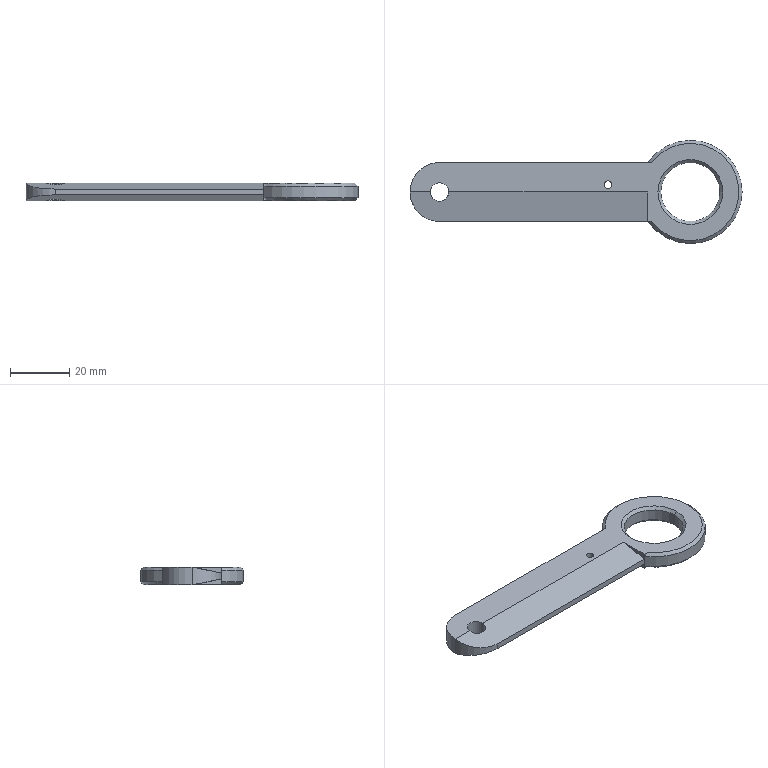Part | SolidWorks | features ICE 3, Chamfer 1, Extrusion 1, HoleWzd 1 | 1 solid | 24 faces | box 112.5 x 35 x 6 mm | volume 11153 mm3 | cylinder 9 | plane 8 | cone 7 | commonest cylinder face diameters 20 x4 2.5 x2 6.2 x2 35 x1
STEP:
#1=CARTESIAN_POINT('',(13.362,2.5,6.));
#2=VERTEX_POINT('',#1);
#3=CARTESIAN_POINT('',(15.862,2.5,6.));
#4=VERTEX_POINT('',#3);
#5=CARTESIAN_POINT('',(14.612,2.5,6.));
#6=DIRECTION('',(0.,0.,1.));
#7=DIRECTION('',(1.,0.,0.));
#8=AXIS2_PLACEMENT_3D('',#5,#6,#7);
#9=CIRCLE('',#8,1.25);
#10=EDGE_CURVE('',#2,#4,#9,.T.);
#11=ORIENTED_EDGE('',*,*,#10,.T.);
#12=CARTESIAN_POINT('',(15.862,2.5,0.));
#13=VERTEX_POINT('',#12);
#14=CARTESIAN_POINT('',(15.862,2.5,0.));
#15=DIRECTION('',(0.,0.,-1.));
#16=VECTOR('',#15,1000.);
#17=LINE('',#14,#16);
#18=EDGE_CURVE('',#4,#13,#17,.T.);
#19=ORIENTED_EDGE('',*,*,#18,.T.);
#20=CARTESIAN_POINT('',(13.362,2.5,0.));
#21=VERTEX_POINT('',#20);
#22=CARTESIAN_POINT('',(14.612,2.5,0.));
#23=DIRECTION('',(0.,0.,-1.));
#24=DIRECTION('',(-1.,0.,0.));
#25=AXIS2_PLACEMENT_3D('',#22,#23,#24);
#26=CIRCLE('',#25,1.25);
#27=EDGE_CURVE('',#13,#21,#26,.T.);
#28=ORIENTED_EDGE('',*,*,#27,.T.);
#29=CARTESIAN_POINT('',(13.362,2.5,0.));
#30=DIRECTION('',(0.,0.,-1.));
#31=VECTOR('',#30,1000.);
#32=LINE('',#29,#31);
#33=EDGE_CURVE('',#2,#21,#32,.T.);
#34=ORIENTED_EDGE('',*,*,#33,.F.);
#35=EDGE_LOOP('',(#11,#19,#28,#34));
#36=FACE_OUTER_BOUND('',#35,.T.);
#37=CARTESIAN_POINT('',(14.612,2.5,0.));
#38=DIRECTION('',(0.,0.,-1.));
#39=DIRECTION('',(-1.,0.,0.));
#40=AXIS2_PLACEMENT_3D('',#37,#38,#39);
#41=CYLINDRICAL_SURFACE('',#40,1.25);
#42=ADVANCED_FACE('',(#36),#41,.F.);
#43=CARTESIAN_POINT('',(52.5,0.,1.));
#44=VERTEX_POINT('',#43);
#45=CARTESIAN_POINT('',(32.5,0.,1.));
#46=VERTEX_POINT('',#45);
#47=CARTESIAN_POINT('',(42.5,0.,1.));
#48=DIRECTION('',(0.,0.,-1.));
#49=DIRECTION('',(1.,0.,0.));
#50=AXIS2_PLACEMENT_3D('',#47,#48,#49);
#51=CIRCLE('',#50,10.);
#52=EDGE_CURVE('',#44,#46,#51,.T.);
#53=ORIENTED_EDGE('',*,*,#52,.F.);
#54=CARTESIAN_POINT('',(53.5,0.,0.));
#55=VERTEX_POINT('',#54);
#56=CARTESIAN_POINT('',(52.5,0.,1.));
#57=DIRECTION('',(0.7071,0.,-0.7071));
#58=VECTOR('',#57,1000.);
#59=LINE('',#56,#58);
#60=EDGE_CURVE('',#44,#55,#59,.T.);
#61=ORIENTED_EDGE('',*,*,#60,.T.);
#62=CARTESIAN_POINT('',(31.5,0.,0.));
#63=VERTEX_POINT('',#62);
#64=CARTESIAN_POINT('',(42.5,0.,0.));
#65=DIRECTION('',(0.,0.,1.));
#66=DIRECTION('',(1.,0.,0.));
#67=AXIS2_PLACEMENT_3D('',#64,#65,#66);
#68=CIRCLE('',#67,11.);
#69=EDGE_CURVE('',#63,#55,#68,.T.);
#70=ORIENTED_EDGE('',*,*,#69,.F.);
#71=CARTESIAN_POINT('',(32.5,0.,1.));
#72=DIRECTION('',(-0.7071,0.,-0.7071));
#73=VECTOR('',#72,1000.);
#74=LINE('',#71,#73);
#75=EDGE_CURVE('',#46,#63,#74,.T.);
#76=ORIENTED_EDGE('',*,*,#75,.F.);
#77=EDGE_LOOP('',(#53,#61,#70,#76));
#78=FACE_OUTER_BOUND('',#77,.T.);
#79=CARTESIAN_POINT('',(42.5,0.,1.));
#80=DIRECTION('',(0.,0.,-1.));
#81=DIRECTION('',(-1.,0.,0.));
#82=AXIS2_PLACEMENT_3D('',#79,#80,#81);
#83=CONICAL_SURFACE('',#82,10.,0.7854);
#84=ADVANCED_FACE('',(#78),#83,.F.);
#85=CARTESIAN_POINT('',(59.,0.,0.));
#86=VERTEX_POINT('',#85);
#87=CARTESIAN_POINT('',(29.376,-10.,0.));
#88=VERTEX_POINT('',#87);
#89=CARTESIAN_POINT('',(42.5,0.,0.));
#90=DIRECTION('',(0.,0.,-1.));
#91=DIRECTION('',(1.,0.,0.));
#92=AXIS2_PLACEMENT_3D('',#89,#90,#91);
#93=CIRCLE('',#92,16.5);
#94=EDGE_CURVE('',#86,#88,#93,.T.);
#95=ORIENTED_EDGE('',*,*,#94,.F.);
#96=CARTESIAN_POINT('',(60.,0.,1.));
#97=VERTEX_POINT('',#96);
#98=CARTESIAN_POINT('',(60.,0.,1.));
#99=DIRECTION('',(0.7071,0.,0.7071));
#100=VECTOR('',#99,1000.);
#101=LINE('',#98,#100);
#102=EDGE_CURVE('',#86,#97,#101,.T.);
#103=ORIENTED_EDGE('',*,*,#102,.T.);
#104=CARTESIAN_POINT('',(28.139,-10.,1.));
#105=VERTEX_POINT('',#104);
#106=CARTESIAN_POINT('',(42.5,0.,1.));
#107=DIRECTION('',(0.,0.,1.));
#108=DIRECTION('',(1.,0.,0.));
#109=AXIS2_PLACEMENT_3D('',#106,#107,#108);
#110=CIRCLE('',#109,17.5);
#111=EDGE_CURVE('',#105,#97,#110,.T.);
#112=ORIENTED_EDGE('',*,*,#111,.F.);
#113=CARTESIAN_POINT('',(29.376,-10.,0.));
#114=CARTESIAN_POINT('',(28.961,-10.,0.3301));
#115=CARTESIAN_POINT('',(28.548,-10.,0.6636));
#116=CARTESIAN_POINT('',(28.139,-10.,1.));
#117=B_SPLINE_CURVE_WITH_KNOTS('',3,(#113,#114,#115,#116),.UNSPECIFIED.,.F.,.F.,(4,4),(0.,0.001591),.UNSPECIFIED.);
#118=EDGE_CURVE('',#88,#105,#117,.T.);
#119=ORIENTED_EDGE('',*,*,#118,.F.);
#120=EDGE_LOOP('',(#95,#103,#112,#119));
#121=FACE_OUTER_BOUND('',#120,.T.);
#122=CARTESIAN_POINT('',(42.5,0.,1.));
#123=DIRECTION('',(0.,0.,1.));
#124=DIRECTION('',(1.,0.,0.));
#125=AXIS2_PLACEMENT_3D('',#122,#123,#124);
#126=CONICAL_SURFACE('',#125,17.5,0.7854);
#127=ADVANCED_FACE('',(#121),#126,.T.);
#128=CARTESIAN_POINT('',(32.5,0.,5.));
#129=VERTEX_POINT('',#128);
#130=CARTESIAN_POINT('',(52.5,0.,5.));
#131=VERTEX_POINT('',#130);
#132=CARTESIAN_POINT('',(42.5,0.,5.));
#133=DIRECTION('',(0.,0.,1.));
#134=DIRECTION('',(1.,0.,0.));
#135=AXIS2_PLACEMENT_3D('',#132,#133,#134);
#136=CIRCLE('',#135,10.);
#137=EDGE_CURVE('',#129,#131,#136,.T.);
#138=ORIENTED_EDGE('',*,*,#137,.F.);
#139=CARTESIAN_POINT('',(31.5,0.,6.));
#140=VERTEX_POINT('',#139);
#141=CARTESIAN_POINT('',(32.5,0.,5.));
#142=DIRECTION('',(-0.7071,0.,0.7071));
#143=VECTOR('',#142,1000.);
#144=LINE('',#141,#143);
#145=EDGE_CURVE('',#129,#140,#144,.T.);
#146=ORIENTED_EDGE('',*,*,#145,.T.);
#147=CARTESIAN_POINT('',(53.5,0.,6.));
#148=VERTEX_POINT('',#147);
#149=CARTESIAN_POINT('',(42.5,0.,6.));
#150=DIRECTION('',(0.,0.,-1.));
#151=DIRECTION('',(1.,0.,0.));
#152=AXIS2_PLACEMENT_3D('',#149,#150,#151);
#153=CIRCLE('',#152,11.);
#154=EDGE_CURVE('',#148,#140,#153,.T.);
#155=ORIENTED_EDGE('',*,*,#154,.F.);
#156=CARTESIAN_POINT('',(52.5,0.,5.));
#157=DIRECTION('',(0.7071,0.,0.7071));
#158=VECTOR('',#157,1000.);
#159=LINE('',#156,#158);
#160=EDGE_CURVE('',#131,#148,#159,.T.);
#161=ORIENTED_EDGE('',*,*,#160,.F.);
#162=EDGE_LOOP('',(#138,#146,#155,#161));
#163=FACE_OUTER_BOUND('',#162,.T.);
#164=CARTESIAN_POINT('',(42.5,0.,5.));
#165=DIRECTION('',(0.,0.,1.));
#166=DIRECTION('',(1.,0.,0.));
#167=AXIS2_PLACEMENT_3D('',#164,#165,#166);
#168=CONICAL_SURFACE('',#167,10.,0.7854);
#169=ADVANCED_FACE('',(#163),#168,.F.);
#170=CARTESIAN_POINT('',(-45.6,0.,6.));
#171=VERTEX_POINT('',#170);
#172=CARTESIAN_POINT('',(-39.4,0.,6.));
#173=VERTEX_POINT('',#172);
#174=CARTESIAN_POINT('',(-45.6,0.,6.));
#175=CARTESIAN_POINT('',(-45.6,-6.2,4.76));
#176=CARTESIAN_POINT('',(-39.4,-6.2,4.76));
#177=CARTESIAN_POINT('',(-39.4,0.,6.));
#178=(BOUNDED_CURVE()B_SPLINE_CURVE(3,(#174,#175,#176,#177),.UNSPECIFIED.,.F.,.F.)B_SPLINE_CURVE_WITH_KNOTS((4,4),(4.712,7.854),.UNSPECIFIED.)CURVE()GEOMETRIC_REPRESENTATION_ITEM()RATIONAL_B_SPLINE_CURVE((1.,0.3333,0.3333,1.))REPRESENTATION_ITEM(''));
#179=EDGE_CURVE('',#171,#173,#178,.T.);
#180=ORIENTED_EDGE('',*,*,#179,.T.);
#181=CARTESIAN_POINT('',(-39.4,0.,0.));
#182=VERTEX_POINT('',#181);
#183=CARTESIAN_POINT('',(-39.4,0.,10.));
#184=DIRECTION('',(0.,0.,-1.));
#185=VECTOR('',#184,1000.);
#186=LINE('',#183,#185);
#187=EDGE_CURVE('',#173,#182,#186,.T.);
#188=ORIENTED_EDGE('',*,*,#187,.T.);
#189=CARTESIAN_POINT('',(-45.6,0.,0.));
#190=VERTEX_POINT('',#189);
#191=CARTESIAN_POINT('',(-39.4,0.,0.));
#192=CARTESIAN_POINT('',(-39.4,-6.2,1.24));
#193=CARTESIAN_POINT('',(-45.6,-6.2,1.24));
#194=CARTESIAN_POINT('',(-45.6,0.,0.));
#195=(BOUNDED_CURVE()B_SPLINE_CURVE(3,(#191,#192,#193,#194),.UNSPECIFIED.,.F.,.F.)B_SPLINE_CURVE_WITH_KNOTS((4,4),(1.571,4.712),.UNSPECIFIED.)CURVE()GEOMETRIC_REPRESENTATION_ITEM()RATIONAL_B_SPLINE_CURVE((1.,0.3333,0.3333,1.))REPRESENTATION_ITEM(''));
#196=EDGE_CURVE('',#182,#190,#195,.T.);
#197=ORIENTED_EDGE('',*,*,#196,.T.);
#198=CARTESIAN_POINT('',(-45.6,0.,10.));
#199=DIRECTION('',(0.,0.,-1.));
#200=VECTOR('',#199,1000.);
#201=LINE('',#198,#200);
#202=EDGE_CURVE('',#171,#190,#201,.T.);
#203=ORIENTED_EDGE('',*,*,#202,.F.);
#204=EDGE_LOOP('',(#180,#188,#197,#203));
#205=FACE_OUTER_BOUND('',#204,.T.);
#206=CARTESIAN_POINT('',(-42.5,0.,10.));
#207=DIRECTION('',(0.,0.,-1.));
#208=DIRECTION('',(-1.,0.,0.));
#209=AXIS2_PLACEMENT_3D('',#206,#207,#208);
#210=CYLINDRICAL_SURFACE('',#209,3.1);
#211=ADVANCED_FACE('',(#205),#210,.F.);
#212=ORIENTED_EDGE('',*,*,#137,.T.);
#213=CARTESIAN_POINT('',(52.5,0.,10.));
#214=DIRECTION('',(0.,0.,-1.));
#215=VECTOR('',#214,1000.);
#216=LINE('',#213,#215);
#217=EDGE_CURVE('',#131,#44,#216,.T.);
#218=ORIENTED_EDGE('',*,*,#217,.T.);
#219=ORIENTED_EDGE('',*,*,#52,.T.);
#220=CARTESIAN_POINT('',(32.5,0.,10.));
#221=DIRECTION('',(0.,0.,-1.));
#222=VECTOR('',#221,1000.);
#223=LINE('',#220,#222);
#224=EDGE_CURVE('',#129,#46,#223,.T.);
#225=ORIENTED_EDGE('',*,*,#224,.F.);
#226=EDGE_LOOP('',(#212,#218,#219,#225));
#227=FACE_OUTER_BOUND('',#226,.T.);
#228=CARTESIAN_POINT('',(42.5,0.,10.));
#229=DIRECTION('',(0.,0.,-1.));
#230=DIRECTION('',(-1.,0.,0.));
#231=AXIS2_PLACEMENT_3D('',#228,#229,#230);
#232=CYLINDRICAL_SURFACE('',#231,10.);
#233=ADVANCED_FACE('',(#227),#232,.F.);
#234=CARTESIAN_POINT('',(-42.5,-10.,4.));
#235=VERTEX_POINT('',#234);
#236=CARTESIAN_POINT('',(-52.5,0.,6.));
#237=VERTEX_POINT('',#236);
#238=CARTESIAN_POINT('',(-42.5,-10.,4.));
#239=CARTESIAN_POINT('',(-48.358,-10.,4.));
#240=CARTESIAN_POINT('',(-52.5,-5.858,4.828));
#241=CARTESIAN_POINT('',(-52.5,0.,6.));
#242=(BOUNDED_CURVE()B_SPLINE_CURVE(3,(#238,#239,#240,#241),.UNSPECIFIED.,.F.,.F.)B_SPLINE_CURVE_WITH_KNOTS((4,4),(0.,1.571),.UNSPECIFIED.)CURVE()GEOMETRIC_REPRESENTATION_ITEM()RATIONAL_B_SPLINE_CURVE((1.,0.8047,0.8047,1.))REPRESENTATION_ITEM(''));
#243=EDGE_CURVE('',#235,#237,#242,.T.);
#244=ORIENTED_EDGE('',*,*,#243,.T.);
#245=CARTESIAN_POINT('',(-52.5,0.,0.));
#246=VERTEX_POINT('',#245);
#247=CARTESIAN_POINT('',(-52.5,0.,6.));
#248=DIRECTION('',(0.,0.,-1.));
#249=VECTOR('',#248,1000.);
#250=LINE('',#247,#249);
#251=EDGE_CURVE('',#237,#246,#250,.T.);
#252=ORIENTED_EDGE('',*,*,#251,.T.);
#253=CARTESIAN_POINT('',(-42.5,-10.,2.));
#254=VERTEX_POINT('',#253);
#255=CARTESIAN_POINT('',(-52.5,0.,0.));
#256=CARTESIAN_POINT('',(-52.5,-5.858,1.172));
#257=CARTESIAN_POINT('',(-48.358,-10.,2.));
#258=CARTESIAN_POINT('',(-42.5,-10.,2.));
#259=(BOUNDED_CURVE()B_SPLINE_CURVE(3,(#255,#256,#257,#258),.UNSPECIFIED.,.F.,.F.)B_SPLINE_CURVE_WITH_KNOTS((4,4),(1.571,3.142),.UNSPECIFIED.)CURVE()GEOMETRIC_REPRESENTATION_ITEM()RATIONAL_B_SPLINE_CURVE((1.,0.8047,0.8047,1.))REPRESENTATION_ITEM(''));
#260=EDGE_CURVE('',#246,#254,#259,.T.);
#261=ORIENTED_EDGE('',*,*,#260,.T.);
#262=CARTESIAN_POINT('',(-42.5,-10.,6.));
#263=DIRECTION('',(0.,0.,-1.));
#264=VECTOR('',#263,1000.);
#265=LINE('',#262,#264);
#266=EDGE_CURVE('',#235,#254,#265,.T.);
#267=ORIENTED_EDGE('',*,*,#266,.F.);
#268=EDGE_LOOP('',(#244,#252,#261,#267));
#269=FACE_OUTER_BOUND('',#268,.T.);
#270=CARTESIAN_POINT('',(-42.5,0.,6.));
#271=DIRECTION('',(0.,0.,-1.));
#272=DIRECTION('',(-1.,0.,0.));
#273=AXIS2_PLACEMENT_3D('',#270,#271,#272);
#274=CYLINDRICAL_SURFACE('',#273,10.);
#275=ADVANCED_FACE('',(#269),#274,.T.);
#276=CARTESIAN_POINT('',(28.,-10.,6.));
#277=VERTEX_POINT('',#276);
#278=CARTESIAN_POINT('',(28.,-10.,4.));
#279=VERTEX_POINT('',#278);
#280=CARTESIAN_POINT('',(28.,-10.,6.));
#281=DIRECTION('',(0.,0.,-1.));
#282=VECTOR('',#281,1000.);
#283=LINE('',#280,#282);
#284=EDGE_CURVE('',#277,#279,#283,.T.);
#285=ORIENTED_EDGE('',*,*,#284,.T.);
#286=CARTESIAN_POINT('',(-52.5,-10.,4.));
#287=DIRECTION('',(1.,0.,0.));
#288=VECTOR('',#287,1000.);
#289=LINE('',#286,#288);
#290=EDGE_CURVE('',#235,#279,#289,.T.);
#291=ORIENTED_EDGE('',*,*,#290,.F.);
#292=ORIENTED_EDGE('',*,*,#266,.T.);
#293=CARTESIAN_POINT('',(28.,-10.,2.));
#294=VERTEX_POINT('',#293);
#295=CARTESIAN_POINT('',(-52.5,-10.,2.));
#296=DIRECTION('',(1.,0.,0.));
#297=VECTOR('',#296,1000.);
#298=LINE('',#295,#297);
#299=EDGE_CURVE('',#254,#294,#298,.T.);
#300=ORIENTED_EDGE('',*,*,#299,.T.);
#301=CARTESIAN_POINT('',(28.,-10.,0.));
#302=VERTEX_POINT('',#301);
#303=CARTESIAN_POINT('',(28.,-10.,0.));
#304=DIRECTION('',(0.,0.,-1.));
#305=VECTOR('',#304,1000.);
#306=LINE('',#303,#305);
#307=EDGE_CURVE('',#294,#302,#306,.T.);
#308=ORIENTED_EDGE('',*,*,#307,.T.);
#309=CARTESIAN_POINT('',(0.,-10.,0.));
#310=DIRECTION('',(1.,0.,0.));
#311=VECTOR('',#310,1000.);
#312=LINE('',#309,#311);
#313=EDGE_CURVE('',#302,#88,#312,.T.);
#314=ORIENTED_EDGE('',*,*,#313,.T.);
#315=ORIENTED_EDGE('',*,*,#118,.T.);
#316=CARTESIAN_POINT('',(28.139,-10.,5.));
#317=VERTEX_POINT('',#316);
#318=CARTESIAN_POINT('',(28.139,-10.,6.));
#319=DIRECTION('',(0.,0.,-1.));
#320=VECTOR('',#319,1000.);
#321=LINE('',#318,#320);
#322=EDGE_CURVE('',#317,#105,#321,.T.);
#323=ORIENTED_EDGE('',*,*,#322,.F.);
#324=CARTESIAN_POINT('',(29.376,-10.,6.));
#325=VERTEX_POINT('',#324);
#326=CARTESIAN_POINT('',(28.139,-10.,5.));
#327=CARTESIAN_POINT('',(28.548,-10.,5.336));
#328=CARTESIAN_POINT('',(28.961,-10.,5.67));
#329=CARTESIAN_POINT('',(29.376,-10.,6.));
#330=B_SPLINE_CURVE_WITH_KNOTS('',3,(#326,#327,#328,#329),.UNSPECIFIED.,.F.,.F.,(4,4),(0.,0.001591),.UNSPECIFIED.);
#331=EDGE_CURVE('',#317,#325,#330,.T.);
#332=ORIENTED_EDGE('',*,*,#331,.T.);
#333=CARTESIAN_POINT('',(0.,-10.,6.));
#334=DIRECTION('',(1.,0.,0.));
#335=VECTOR('',#334,1000.);
#336=LINE('',#333,#335);
#337=EDGE_CURVE('',#277,#325,#336,.T.);
#338=ORIENTED_EDGE('',*,*,#337,.F.);
#339=EDGE_LOOP('',(#285,#291,#292,#300,#308,#314,#315,#323,#332,#338));
#340=FACE_OUTER_BOUND('',#339,.T.);
#341=CARTESIAN_POINT('',(0.,-10.,6.));
#342=DIRECTION('',(0.,1.,0.));
#343=DIRECTION('',(0.,0.,1.));
#344=AXIS2_PLACEMENT_3D('',#341,#342,#343);
#345=PLANE('',#344);
#346=ADVANCED_FACE('',(#340),#345,.F.);
#347=CARTESIAN_POINT('',(28.139,10.,5.));
#348=VERTEX_POINT('',#347);
#349=CARTESIAN_POINT('',(28.139,10.,1.));
#350=VERTEX_POINT('',#349);
#351=CARTESIAN_POINT('',(28.139,10.,6.));
#352=DIRECTION('',(0.,0.,-1.));
#353=VECTOR('',#352,1000.);
#354=LINE('',#351,#353);
#355=EDGE_CURVE('',#348,#350,#354,.T.);
#356=ORIENTED_EDGE('',*,*,#355,.F.);
#357=CARTESIAN_POINT('',(42.5,0.,5.));
#358=DIRECTION('',(0.,0.,-1.));
#359=DIRECTION('',(1.,0.,0.));
#360=AXIS2_PLACEMENT_3D('',#357,#358,#359);
#361=CIRCLE('',#360,17.5);
#362=EDGE_CURVE('',#348,#317,#361,.T.);
#363=ORIENTED_EDGE('',*,*,#362,.T.);
#364=ORIENTED_EDGE('',*,*,#322,.T.);
#365=ORIENTED_EDGE('',*,*,#111,.T.);
#366=CARTESIAN_POINT('',(42.5,0.,1.));
#367=DIRECTION('',(0.,0.,1.));
#368=DIRECTION('',(1.,0.,0.));
#369=AXIS2_PLACEMENT_3D('',#366,#367,#368);
#370=CIRCLE('',#369,17.5);
#371=EDGE_CURVE('',#97,#350,#370,.T.);
#372=ORIENTED_EDGE('',*,*,#371,.T.);
#373=EDGE_LOOP('',(#356,#363,#364,#365,#372));
#374=FACE_OUTER_BOUND('',#373,.T.);
#375=CARTESIAN_POINT('',(42.5,0.,6.));
#376=DIRECTION('',(0.,0.,-1.));
#377=DIRECTION('',(-1.,0.,0.));
#378=AXIS2_PLACEMENT_3D('',#375,#376,#377);
#379=CYLINDRICAL_SURFACE('',#378,17.5);
#380=ADVANCED_FACE('',(#374),#379,.T.);
#381=CARTESIAN_POINT('',(-42.5,10.,0.));
#382=VERTEX_POINT('',#381);
#383=CARTESIAN_POINT('',(29.376,10.,0.));
#384=VERTEX_POINT('',#383);
#385=CARTESIAN_POINT('',(0.,10.,0.));
#386=DIRECTION('',(1.,0.,0.));
#387=VECTOR('',#386,1000.);
#388=LINE('',#385,#387);
#389=EDGE_CURVE('',#382,#384,#388,.T.);
#390=ORIENTED_EDGE('',*,*,#389,.F.);
#391=CARTESIAN_POINT('',(-42.5,10.,6.));
#392=VERTEX_POINT('',#391);
#393=CARTESIAN_POINT('',(-42.5,10.,6.));
#394=DIRECTION('',(0.,0.,-1.));
#395=VECTOR('',#394,1000.);
#396=LINE('',#393,#395);
#397=EDGE_CURVE('',#392,#382,#396,.T.);
#398=ORIENTED_EDGE('',*,*,#397,.F.);
#399=CARTESIAN_POINT('',(29.376,10.,6.));
#400=VERTEX_POINT('',#399);
#401=CARTESIAN_POINT('',(0.,10.,6.));
#402=DIRECTION('',(1.,0.,0.));
#403=VECTOR('',#402,1000.);
#404=LINE('',#401,#403);
#405=EDGE_CURVE('',#392,#400,#404,.T.);
#406=ORIENTED_EDGE('',*,*,#405,.T.);
#407=CARTESIAN_POINT('',(29.376,10.,6.));
#408=CARTESIAN_POINT('',(28.961,10.,5.67));
#409=CARTESIAN_POINT('',(28.548,10.,5.336));
#410=CARTESIAN_POINT('',(28.139,10.,5.));
#411=B_SPLINE_CURVE_WITH_KNOTS('',3,(#407,#408,#409,#410),.UNSPECIFIED.,.F.,.F.,(4,4),(0.,0.001591),.UNSPECIFIED.);
#412=EDGE_CURVE('',#400,#348,#411,.T.);
#413=ORIENTED_EDGE('',*,*,#412,.T.);
#414=ORIENTED_EDGE('',*,*,#355,.T.);
#415=CARTESIAN_POINT('',(28.139,10.,1.));
#416=CARTESIAN_POINT('',(28.548,10.,0.6636));
#417=CARTESIAN_POINT('',(28.961,10.,0.3301));
#418=CARTESIAN_POINT('',(29.376,10.,0.));
#419=B_SPLINE_CURVE_WITH_KNOTS('',3,(#415,#416,#417,#418),.UNSPECIFIED.,.F.,.F.,(4,4),(0.,0.001591),.UNSPECIFIED.);
#420=EDGE_CURVE('',#350,#384,#419,.T.);
#421=ORIENTED_EDGE('',*,*,#420,.T.);
#422=EDGE_LOOP('',(#390,#398,#406,#413,#414,#421));
#423=FACE_OUTER_BOUND('',#422,.T.);
#424=CARTESIAN_POINT('',(0.,10.,6.));
#425=DIRECTION('',(0.,1.,0.));
#426=DIRECTION('',(0.,0.,1.));
#427=AXIS2_PLACEMENT_3D('',#424,#425,#426);
#428=PLANE('',#427);
#429=ADVANCED_FACE('',(#423),#428,.T.);
#430=ORIENTED_EDGE('',*,*,#251,.F.);
#431=CARTESIAN_POINT('',(-42.5,0.,6.));
#432=DIRECTION('',(0.,0.,1.));
#433=DIRECTION('',(1.,0.,0.));
#434=AXIS2_PLACEMENT_3D('',#431,#432,#433);
#435=CIRCLE('',#434,10.);
#436=EDGE_CURVE('',#392,#237,#435,.T.);
#437=ORIENTED_EDGE('',*,*,#436,.F.);
#438=ORIENTED_EDGE('',*,*,#397,.T.);
#439=CARTESIAN_POINT('',(-42.5,0.,0.));
#440=DIRECTION('',(0.,0.,1.));
#441=DIRECTION('',(1.,0.,0.));
#442=AXIS2_PLACEMENT_3D('',#439,#440,#441);
#443=CIRCLE('',#442,10.);
#444=EDGE_CURVE('',#382,#246,#443,.T.);
#445=ORIENTED_EDGE('',*,*,#444,.T.);
#446=EDGE_LOOP('',(#430,#437,#438,#445));
#447=FACE_OUTER_BOUND('',#446,.T.);
#448=CARTESIAN_POINT('',(-42.5,0.,6.));
#449=DIRECTION('',(0.,0.,-1.));
#450=DIRECTION('',(-1.,0.,0.));
#451=AXIS2_PLACEMENT_3D('',#448,#449,#450);
#452=CYLINDRICAL_SURFACE('',#451,10.);
#453=ADVANCED_FACE('',(#447),#452,.T.);
#454=ORIENTED_EDGE('',*,*,#10,.F.);
#455=CARTESIAN_POINT('',(14.612,2.5,6.));
#456=DIRECTION('',(0.,0.,1.));
#457=DIRECTION('',(1.,0.,0.));
#458=AXIS2_PLACEMENT_3D('',#455,#456,#457);
#459=CIRCLE('',#458,1.25);
#460=EDGE_CURVE('',#4,#2,#459,.T.);
#461=ORIENTED_EDGE('',*,*,#460,.F.);
#462=EDGE_LOOP('',(#454,#461));
#463=FACE_BOUND('',#462,.T.);
#464=ORIENTED_EDGE('',*,*,#154,.T.);
#465=CARTESIAN_POINT('',(42.5,0.,6.));
#466=DIRECTION('',(0.,0.,-1.));
#467=DIRECTION('',(1.,0.,0.));
#468=AXIS2_PLACEMENT_3D('',#465,#466,#467);
#469=CIRCLE('',#468,11.);
#470=EDGE_CURVE('',#140,#148,#469,.T.);
#471=ORIENTED_EDGE('',*,*,#470,.T.);
#472=EDGE_LOOP('',(#464,#471));
#473=FACE_BOUND('',#472,.T.);
#474=CARTESIAN_POINT('',(42.5,0.,6.));
#475=DIRECTION('',(0.,0.,1.));
#476=DIRECTION('',(1.,0.,0.));
#477=AXIS2_PLACEMENT_3D('',#474,#475,#476);
#478=CIRCLE('',#477,16.5);
#479=EDGE_CURVE('',#325,#400,#478,.T.);
#480=ORIENTED_EDGE('',*,*,#479,.T.);
#481=ORIENTED_EDGE('',*,*,#405,.F.);
#482=ORIENTED_EDGE('',*,*,#436,.T.);
#483=CARTESIAN_POINT('',(-52.5,0.,6.));
#484=DIRECTION('',(1.,0.,0.));
#485=VECTOR('',#484,1000.);
#486=LINE('',#483,#485);
#487=EDGE_CURVE('',#237,#171,#486,.T.);
#488=ORIENTED_EDGE('',*,*,#487,.T.);
#489=CARTESIAN_POINT('',(-42.5,0.,6.));
#490=DIRECTION('',(0.,0.,1.));
#491=DIRECTION('',(1.,0.,0.));
#492=AXIS2_PLACEMENT_3D('',#489,#490,#491);
#493=CIRCLE('',#492,3.1);
#494=EDGE_CURVE('',#173,#171,#493,.T.);
#495=ORIENTED_EDGE('',*,*,#494,.F.);
#496=CARTESIAN_POINT('',(28.,0.,6.));
#497=VERTEX_POINT('',#496);
#498=CARTESIAN_POINT('',(-52.5,0.,6.));
#499=DIRECTION('',(1.,0.,0.));
#500=VECTOR('',#499,1000.);
#501=LINE('',#498,#500);
#502=EDGE_CURVE('',#173,#497,#501,.T.);
#503=ORIENTED_EDGE('',*,*,#502,.T.);
#504=CARTESIAN_POINT('',(28.,0.,6.));
#505=DIRECTION('',(0.,-1.,0.));
#506=VECTOR('',#505,1000.);
#507=LINE('',#504,#506);
#508=EDGE_CURVE('',#497,#277,#507,.T.);
#509=ORIENTED_EDGE('',*,*,#508,.T.);
#510=ORIENTED_EDGE('',*,*,#337,.T.);
#511=EDGE_LOOP('',(#480,#481,#482,#488,#495,#503,#509,#510));
#512=FACE_OUTER_BOUND('',#511,.T.);
#513=CARTESIAN_POINT('',(0.,0.,6.));
#514=DIRECTION('',(0.,0.,1.));
#515=DIRECTION('',(1.,0.,0.));
#516=AXIS2_PLACEMENT_3D('',#513,#514,#515);
#517=PLANE('',#516);
#518=ADVANCED_FACE('',(#463,#473,#512),#517,.T.);
#519=CARTESIAN_POINT('',(14.612,2.5,0.));
#520=DIRECTION('',(0.,0.,-1.));
#521=DIRECTION('',(-1.,0.,0.));
#522=AXIS2_PLACEMENT_3D('',#519,#520,#521);
#523=CIRCLE('',#522,1.25);
#524=EDGE_CURVE('',#21,#13,#523,.T.);
#525=ORIENTED_EDGE('',*,*,#524,.F.);
#526=ORIENTED_EDGE('',*,*,#27,.F.);
#527=EDGE_LOOP('',(#525,#526));
#528=FACE_BOUND('',#527,.T.);
#529=ORIENTED_EDGE('',*,*,#69,.T.);
#530=CARTESIAN_POINT('',(42.5,0.,0.));
#531=DIRECTION('',(0.,0.,1.));
#532=DIRECTION('',(1.,0.,0.));
#533=AXIS2_PLACEMENT_3D('',#530,#531,#532);
#534=CIRCLE('',#533,11.);
#535=EDGE_CURVE('',#55,#63,#534,.T.);
#536=ORIENTED_EDGE('',*,*,#535,.T.);
#537=EDGE_LOOP('',(#529,#536));
#538=FACE_BOUND('',#537,.T.);
#539=ORIENTED_EDGE('',*,*,#389,.T.);
#540=CARTESIAN_POINT('',(42.5,0.,0.));
#541=DIRECTION('',(0.,0.,-1.));
#542=DIRECTION('',(1.,0.,0.));
#543=AXIS2_PLACEMENT_3D('',#540,#541,#542);
#544=CIRCLE('',#543,16.5);
#545=EDGE_CURVE('',#384,#86,#544,.T.);
#546=ORIENTED_EDGE('',*,*,#545,.T.);
#547=ORIENTED_EDGE('',*,*,#94,.T.);
#548=ORIENTED_EDGE('',*,*,#313,.F.);
#549=CARTESIAN_POINT('',(28.,0.,0.));
#550=VERTEX_POINT('',#549);
#551=CARTESIAN_POINT('',(28.,0.,0.));
#552=DIRECTION('',(0.,1.,0.));
#553=VECTOR('',#552,1000.);
#554=LINE('',#551,#553);
#555=EDGE_CURVE('',#302,#550,#554,.T.);
#556=ORIENTED_EDGE('',*,*,#555,.T.);
#557=CARTESIAN_POINT('',(-52.5,0.,0.));
#558=DIRECTION('',(1.,0.,0.));
#559=VECTOR('',#558,1000.);
#560=LINE('',#557,#559);
#561=EDGE_CURVE('',#182,#550,#560,.T.);
#562=ORIENTED_EDGE('',*,*,#561,.F.);
#563=CARTESIAN_POINT('',(-42.5,0.,0.));
#564=DIRECTION('',(0.,0.,-1.));
#565=DIRECTION('',(-1.,0.,0.));
#566=AXIS2_PLACEMENT_3D('',#563,#564,#565);
#567=CIRCLE('',#566,3.1);
#568=EDGE_CURVE('',#190,#182,#567,.T.);
#569=ORIENTED_EDGE('',*,*,#568,.F.);
#570=CARTESIAN_POINT('',(-52.5,0.,0.));
#571=DIRECTION('',(1.,0.,0.));
#572=VECTOR('',#571,1000.);
#573=LINE('',#570,#572);
#574=EDGE_CURVE('',#246,#190,#573,.T.);
#575=ORIENTED_EDGE('',*,*,#574,.F.);
#576=ORIENTED_EDGE('',*,*,#444,.F.);
#577=EDGE_LOOP('',(#539,#546,#547,#548,#556,#562,#569,#575,#576));
#578=FACE_OUTER_BOUND('',#577,.T.);
#579=CARTESIAN_POINT('',(0.,0.,0.));
#580=DIRECTION('',(0.,0.,1.));
#581=DIRECTION('',(1.,0.,0.));
#582=AXIS2_PLACEMENT_3D('',#579,#580,#581);
#583=PLANE('',#582);
#584=ADVANCED_FACE('',(#528,#538,#578),#583,.F.);
#585=ORIENTED_EDGE('',*,*,#217,.F.);
#586=CARTESIAN_POINT('',(42.5,0.,5.));
#587=DIRECTION('',(0.,0.,1.));
#588=DIRECTION('',(1.,0.,0.));
#589=AXIS2_PLACEMENT_3D('',#586,#587,#588);
#590=CIRCLE('',#589,10.);
#591=EDGE_CURVE('',#131,#129,#590,.T.);
#592=ORIENTED_EDGE('',*,*,#591,.T.);
#593=ORIENTED_EDGE('',*,*,#224,.T.);
#594=CARTESIAN_POINT('',(42.5,0.,1.));
#595=DIRECTION('',(0.,0.,-1.));
#596=DIRECTION('',(1.,0.,0.));
#597=AXIS2_PLACEMENT_3D('',#594,#595,#596);
#598=CIRCLE('',#597,10.);
#599=EDGE_CURVE('',#46,#44,#598,.T.);
#600=ORIENTED_EDGE('',*,*,#599,.T.);
#601=EDGE_LOOP('',(#585,#592,#593,#600));
#602=FACE_OUTER_BOUND('',#601,.T.);
#603=CARTESIAN_POINT('',(42.5,0.,10.));
#604=DIRECTION('',(0.,0.,-1.));
#605=DIRECTION('',(-1.,0.,0.));
#606=AXIS2_PLACEMENT_3D('',#603,#604,#605);
#607=CYLINDRICAL_SURFACE('',#606,10.);
#608=ADVANCED_FACE('',(#602),#607,.F.);
#609=ORIENTED_EDGE('',*,*,#187,.F.);
#610=ORIENTED_EDGE('',*,*,#494,.T.);
#611=ORIENTED_EDGE('',*,*,#202,.T.);
#612=ORIENTED_EDGE('',*,*,#568,.T.);
#613=EDGE_LOOP('',(#609,#610,#611,#612));
#614=FACE_OUTER_BOUND('',#613,.T.);
#615=CARTESIAN_POINT('',(-42.5,0.,10.));
#616=DIRECTION('',(0.,0.,-1.));
#617=DIRECTION('',(-1.,0.,0.));
#618=AXIS2_PLACEMENT_3D('',#615,#616,#617);
#619=CYLINDRICAL_SURFACE('',#618,3.1);
#620=ADVANCED_FACE('',(#614),#619,.F.);
#621=ORIENTED_EDGE('',*,*,#574,.T.);
#622=ORIENTED_EDGE('',*,*,#196,.F.);
#623=ORIENTED_EDGE('',*,*,#561,.T.);
#624=CARTESIAN_POINT('',(28.,-10.,2.));
#625=DIRECTION('',(0.,-0.9806,0.1961));
#626=VECTOR('',#625,1000.);
#627=LINE('',#624,#626);
#628=EDGE_CURVE('',#550,#294,#627,.T.);
#629=ORIENTED_EDGE('',*,*,#628,.T.);
#630=ORIENTED_EDGE('',*,*,#299,.F.);
#631=ORIENTED_EDGE('',*,*,#260,.F.);
#632=EDGE_LOOP('',(#621,#622,#623,#629,#630,#631));
#633=FACE_OUTER_BOUND('',#632,.T.);
#634=CARTESIAN_POINT('',(-52.5,-10.,2.));
#635=DIRECTION('',(0.,0.1961,0.9806));
#636=DIRECTION('',(0.,-0.9806,0.1961));
#637=AXIS2_PLACEMENT_3D('',#634,#635,#636);
#638=PLANE('',#637);
#639=ADVANCED_FACE('',(#633),#638,.F.);
#640=ORIENTED_EDGE('',*,*,#307,.F.);
#641=ORIENTED_EDGE('',*,*,#628,.F.);
#642=ORIENTED_EDGE('',*,*,#555,.F.);
#643=EDGE_LOOP('',(#640,#641,#642));
#644=FACE_OUTER_BOUND('',#643,.T.);
#645=CARTESIAN_POINT('',(28.,0.,0.));
#646=DIRECTION('',(1.,0.,0.));
#647=DIRECTION('',(0.,0.,-1.));
#648=AXIS2_PLACEMENT_3D('',#645,#646,#647);
#649=PLANE('',#648);
#650=ADVANCED_FACE('',(#644),#649,.F.);
#651=ORIENTED_EDGE('',*,*,#290,.T.);
#652=CARTESIAN_POINT('',(28.,-10.,4.));
#653=DIRECTION('',(0.,0.9806,0.1961));
#654=VECTOR('',#653,1000.);
#655=LINE('',#652,#654);
#656=EDGE_CURVE('',#279,#497,#655,.T.);
#657=ORIENTED_EDGE('',*,*,#656,.T.);
#658=ORIENTED_EDGE('',*,*,#502,.F.);
#659=ORIENTED_EDGE('',*,*,#179,.F.);
#660=ORIENTED_EDGE('',*,*,#487,.F.);
#661=ORIENTED_EDGE('',*,*,#243,.F.);
#662=EDGE_LOOP('',(#651,#657,#658,#659,#660,#661));
#663=FACE_OUTER_BOUND('',#662,.T.);
#664=CARTESIAN_POINT('',(-52.5,-10.,4.));
#665=DIRECTION('',(0.,0.1961,-0.9806));
#666=DIRECTION('',(0.,0.9806,0.1961));
#667=AXIS2_PLACEMENT_3D('',#664,#665,#666);
#668=PLANE('',#667);
#669=ADVANCED_FACE('',(#663),#668,.F.);
#670=ORIENTED_EDGE('',*,*,#284,.F.);
#671=ORIENTED_EDGE('',*,*,#508,.F.);
#672=ORIENTED_EDGE('',*,*,#656,.F.);
#673=EDGE_LOOP('',(#670,#671,#672));
#674=FACE_OUTER_BOUND('',#673,.T.);
#675=CARTESIAN_POINT('',(28.,0.,0.));
#676=DIRECTION('',(-1.,0.,0.));
#677=DIRECTION('',(0.,0.,1.));
#678=AXIS2_PLACEMENT_3D('',#675,#676,#677);
#679=PLANE('',#678);
#680=ADVANCED_FACE('',(#674),#679,.T.);
#681=ORIENTED_EDGE('',*,*,#145,.F.);
#682=ORIENTED_EDGE('',*,*,#591,.F.);
#683=ORIENTED_EDGE('',*,*,#160,.T.);
#684=ORIENTED_EDGE('',*,*,#470,.F.);
#685=EDGE_LOOP('',(#681,#682,#683,#684));
#686=FACE_OUTER_BOUND('',#685,.T.);
#687=CARTESIAN_POINT('',(42.5,0.,5.));
#688=DIRECTION('',(0.,0.,1.));
#689=DIRECTION('',(1.,0.,0.));
#690=AXIS2_PLACEMENT_3D('',#687,#688,#689);
#691=CONICAL_SURFACE('',#690,10.,0.7854);
#692=ADVANCED_FACE('',(#686),#691,.F.);
#693=ORIENTED_EDGE('',*,*,#331,.F.);
#694=ORIENTED_EDGE('',*,*,#362,.F.);
#695=ORIENTED_EDGE('',*,*,#412,.F.);
#696=ORIENTED_EDGE('',*,*,#479,.F.);
#697=EDGE_LOOP('',(#693,#694,#695,#696));
#698=FACE_OUTER_BOUND('',#697,.T.);
#699=CARTESIAN_POINT('',(42.5,0.,6.));
#700=DIRECTION('',(0.,0.,-1.));
#701=DIRECTION('',(-1.,0.,0.));
#702=AXIS2_PLACEMENT_3D('',#699,#700,#701);
#703=CONICAL_SURFACE('',#702,16.5,0.7854);
#704=ADVANCED_FACE('',(#698),#703,.T.);
#705=ORIENTED_EDGE('',*,*,#102,.F.);
#706=ORIENTED_EDGE('',*,*,#545,.F.);
#707=ORIENTED_EDGE('',*,*,#420,.F.);
#708=ORIENTED_EDGE('',*,*,#371,.F.);
#709=EDGE_LOOP('',(#705,#706,#707,#708));
#710=FACE_OUTER_BOUND('',#709,.T.);
#711=CARTESIAN_POINT('',(42.5,0.,1.));
#712=DIRECTION('',(0.,0.,1.));
#713=DIRECTION('',(1.,0.,0.));
#714=AXIS2_PLACEMENT_3D('',#711,#712,#713);
#715=CONICAL_SURFACE('',#714,17.5,0.7854);
#716=ADVANCED_FACE('',(#710),#715,.T.);
#717=ORIENTED_EDGE('',*,*,#60,.F.);
#718=ORIENTED_EDGE('',*,*,#599,.F.);
#719=ORIENTED_EDGE('',*,*,#75,.T.);
#720=ORIENTED_EDGE('',*,*,#535,.F.);
#721=EDGE_LOOP('',(#717,#718,#719,#720));
#722=FACE_OUTER_BOUND('',#721,.T.);
#723=CARTESIAN_POINT('',(42.5,0.,1.));
#724=DIRECTION('',(0.,0.,-1.));
#725=DIRECTION('',(-1.,0.,0.));
#726=AXIS2_PLACEMENT_3D('',#723,#724,#725);
#727=CONICAL_SURFACE('',#726,10.,0.7854);
#728=ADVANCED_FACE('',(#722),#727,.F.);
#729=ORIENTED_EDGE('',*,*,#18,.F.);
#730=ORIENTED_EDGE('',*,*,#460,.T.);
#731=ORIENTED_EDGE('',*,*,#33,.T.);
#732=ORIENTED_EDGE('',*,*,#524,.T.);
#733=EDGE_LOOP('',(#729,#730,#731,#732));
#734=FACE_OUTER_BOUND('',#733,.T.);
#735=CARTESIAN_POINT('',(14.612,2.5,0.));
#736=DIRECTION('',(0.,0.,-1.));
#737=DIRECTION('',(-1.,0.,0.));
#738=AXIS2_PLACEMENT_3D('',#735,#736,#737);
#739=CYLINDRICAL_SURFACE('',#738,1.25);
#740=ADVANCED_FACE('',(#734),#739,.F.);
#741=CLOSED_SHELL('',(#42,#84,#127,#169,#211,#233,#275,#346,#380,#429,#453,#518,#584,#608,#620,#639,#650,#669,#680,#692,#704,#716,#728,#740));
#742=MANIFOLD_SOLID_BREP('',#741);
#743=CARTESIAN_POINT('',(0.,0.,0.));
#744=DIRECTION('',(0.,0.,1.));
#745=DIRECTION('',(1.,0.,0.));
#746=AXIS2_PLACEMENT_3D('',#743,#744,#745);
#747=(LENGTH_UNIT()NAMED_UNIT(*)SI_UNIT(.MILLI.,.METRE.));
#748=UNCERTAINTY_MEASURE_WITH_UNIT(LENGTH_MEASURE(0.00001),#747,'','');
#749=(NAMED_UNIT(*)PLANE_ANGLE_UNIT()SI_UNIT($,.RADIAN.));
#750=(NAMED_UNIT(*)SI_UNIT($,.STERADIAN.)SOLID_ANGLE_UNIT());
#751=(GEOMETRIC_REPRESENTATION_CONTEXT(3)GLOBAL_UNCERTAINTY_ASSIGNED_CONTEXT((#748))GLOBAL_UNIT_ASSIGNED_CONTEXT((#747,#749,#750))REPRESENTATION_CONTEXT('',''));
#752=ADVANCED_BREP_SHAPE_REPRESENTATION('',(#742,#746),#751);